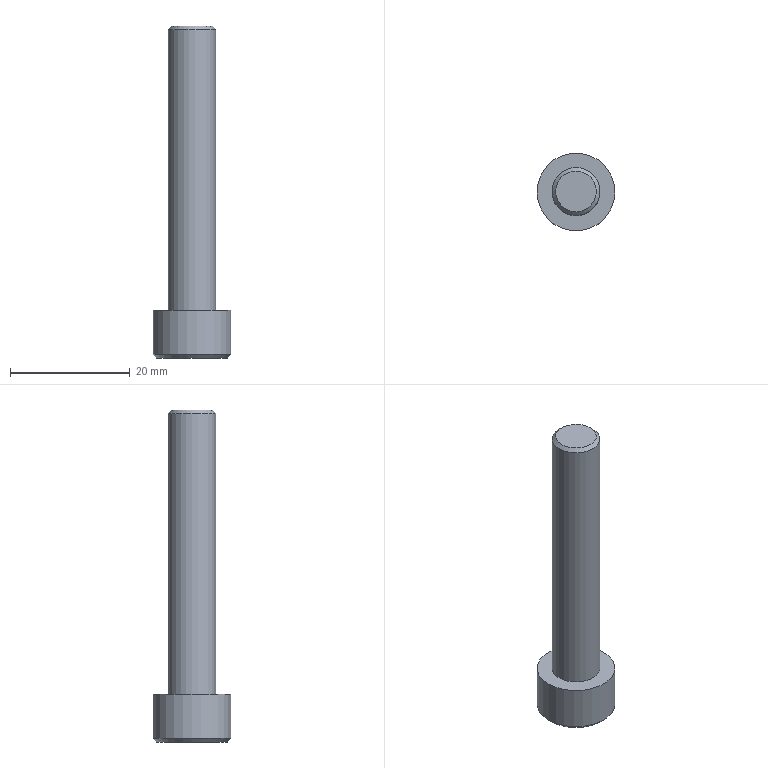Part | NX | features M8.00-55.00 2 | 1 solid | 14 faces | box 13 x 13 x 55.5 mm | volume 3278 mm3 | plane 10 | cylinder 2 | cone 2 | commonest cylinder face diameters 8 x1 13 x1
STEP:
#1=CARTESIAN_POINT('',(19.1,90.,-109.5));
#2=VERTEX_POINT('',#1);
#3=CARTESIAN_POINT('',(25.,90.,-109.5));
#4=DIRECTION('',(0.,0.,-1.));
#5=DIRECTION('',(-1.,0.,0.));
#6=AXIS2_PLACEMENT_3D('',#3,#4,#5);
#7=CIRCLE('',#6,5.9);
#8=EDGE_CURVE('',#2,#2,#7,.T.);
#9=ORIENTED_EDGE('',*,*,#8,.T.);
#10=EDGE_LOOP('',(#9));
#11=FACE_BOUND('',#10,.T.);
#12=CARTESIAN_POINT('',(28.4,91.963,-109.5));
#13=VERTEX_POINT('',#12);
#14=CARTESIAN_POINT('',(28.4,88.037,-109.5));
#15=VERTEX_POINT('',#14);
#16=CARTESIAN_POINT('',(28.4,91.963,-109.5));
#17=DIRECTION('',(0.,-1.,0.));
#18=VECTOR('',#17,1000.);
#19=LINE('',#16,#18);
#20=EDGE_CURVE('',#13,#15,#19,.T.);
#21=ORIENTED_EDGE('',*,*,#20,.F.);
#22=CARTESIAN_POINT('',(25.,93.926,-109.5));
#23=VERTEX_POINT('',#22);
#24=CARTESIAN_POINT('',(25.,93.926,-109.5));
#25=DIRECTION('',(0.866,-0.5,0.));
#26=VECTOR('',#25,1000.);
#27=LINE('',#24,#26);
#28=EDGE_CURVE('',#23,#13,#27,.T.);
#29=ORIENTED_EDGE('',*,*,#28,.F.);
#30=CARTESIAN_POINT('',(21.6,91.963,-109.5));
#31=VERTEX_POINT('',#30);
#32=CARTESIAN_POINT('',(21.6,91.963,-109.5));
#33=DIRECTION('',(0.866,0.5,0.));
#34=VECTOR('',#33,1000.);
#35=LINE('',#32,#34);
#36=EDGE_CURVE('',#31,#23,#35,.T.);
#37=ORIENTED_EDGE('',*,*,#36,.F.);
#38=CARTESIAN_POINT('',(21.6,88.037,-109.5));
#39=VERTEX_POINT('',#38);
#40=CARTESIAN_POINT('',(21.6,88.037,-109.5));
#41=DIRECTION('',(0.,1.,0.));
#42=VECTOR('',#41,1000.);
#43=LINE('',#40,#42);
#44=EDGE_CURVE('',#39,#31,#43,.T.);
#45=ORIENTED_EDGE('',*,*,#44,.F.);
#46=CARTESIAN_POINT('',(25.,86.074,-109.5));
#47=VERTEX_POINT('',#46);
#48=CARTESIAN_POINT('',(25.,86.074,-109.5));
#49=DIRECTION('',(-0.866,0.5,0.));
#50=VECTOR('',#49,1000.);
#51=LINE('',#48,#50);
#52=EDGE_CURVE('',#47,#39,#51,.T.);
#53=ORIENTED_EDGE('',*,*,#52,.F.);
#54=CARTESIAN_POINT('',(28.4,88.037,-109.5));
#55=DIRECTION('',(-0.866,-0.5,0.));
#56=VECTOR('',#55,1000.);
#57=LINE('',#54,#56);
#58=EDGE_CURVE('',#15,#47,#57,.T.);
#59=ORIENTED_EDGE('',*,*,#58,.F.);
#60=EDGE_LOOP('',(#21,#29,#37,#45,#53,#59));
#61=FACE_BOUND('',#60,.T.);
#62=CARTESIAN_POINT('',(25.,90.,-109.5));
#63=DIRECTION('',(0.,0.,-1.));
#64=DIRECTION('',(-1.,0.,0.));
#65=AXIS2_PLACEMENT_3D('',#62,#63,#64);
#66=PLANE('',#65);
#67=ADVANCED_FACE('',(#11,#61),#66,.T.);
#68=CARTESIAN_POINT('',(29.,90.,-101.5));
#69=VERTEX_POINT('',#68);
#70=CARTESIAN_POINT('',(25.,90.,-101.5));
#71=DIRECTION('',(0.,0.,1.));
#72=DIRECTION('',(1.,0.,0.));
#73=AXIS2_PLACEMENT_3D('',#70,#71,#72);
#74=CIRCLE('',#73,4.);
#75=EDGE_CURVE('',#69,#69,#74,.T.);
#76=ORIENTED_EDGE('',*,*,#75,.F.);
#77=EDGE_LOOP('',(#76));
#78=FACE_BOUND('',#77,.T.);
#79=CARTESIAN_POINT('',(31.5,90.,-101.5));
#80=VERTEX_POINT('',#79);
#81=CARTESIAN_POINT('',(25.,90.,-101.5));
#82=DIRECTION('',(0.,0.,-1.));
#83=DIRECTION('',(1.,0.,0.));
#84=AXIS2_PLACEMENT_3D('',#81,#82,#83);
#85=CIRCLE('',#84,6.5);
#86=EDGE_CURVE('',#80,#80,#85,.T.);
#87=ORIENTED_EDGE('',*,*,#86,.F.);
#88=EDGE_LOOP('',(#87));
#89=FACE_BOUND('',#88,.T.);
#90=CARTESIAN_POINT('',(25.,90.,-101.5));
#91=DIRECTION('',(0.,0.,1.));
#92=DIRECTION('',(1.,0.,0.));
#93=AXIS2_PLACEMENT_3D('',#90,#91,#92);
#94=PLANE('',#93);
#95=ADVANCED_FACE('',(#78,#89),#94,.T.);
#96=CARTESIAN_POINT('',(18.5,90.,-108.9));
#97=VERTEX_POINT('',#96);
#98=CARTESIAN_POINT('',(25.,90.,-108.9));
#99=DIRECTION('',(0.,0.,-1.));
#100=DIRECTION('',(-1.,0.,0.));
#101=AXIS2_PLACEMENT_3D('',#98,#99,#100);
#102=CIRCLE('',#101,6.5);
#103=EDGE_CURVE('',#97,#97,#102,.F.);
#104=ORIENTED_EDGE('',*,*,#103,.T.);
#105=EDGE_LOOP('',(#104));
#106=FACE_BOUND('',#105,.T.);
#107=ORIENTED_EDGE('',*,*,#86,.T.);
#108=EDGE_LOOP('',(#107));
#109=FACE_BOUND('',#108,.T.);
#110=CARTESIAN_POINT('',(25.,90.,-101.5));
#111=DIRECTION('',(0.,0.,-1.));
#112=DIRECTION('',(1.,0.,0.));
#113=AXIS2_PLACEMENT_3D('',#110,#111,#112);
#114=CYLINDRICAL_SURFACE('',#113,6.5);
#115=ADVANCED_FACE('',(#106,#109),#114,.T.);
#116=CARTESIAN_POINT('',(28.4,90.,-54.));
#117=VERTEX_POINT('',#116);
#118=CARTESIAN_POINT('',(25.,90.,-54.));
#119=DIRECTION('',(0.,0.,1.));
#120=DIRECTION('',(1.,0.,0.));
#121=AXIS2_PLACEMENT_3D('',#118,#119,#120);
#122=CIRCLE('',#121,3.4);
#123=EDGE_CURVE('',#117,#117,#122,.T.);
#124=ORIENTED_EDGE('',*,*,#123,.T.);
#125=EDGE_LOOP('',(#124));
#126=FACE_BOUND('',#125,.T.);
#127=CARTESIAN_POINT('',(25.,90.,-54.));
#128=DIRECTION('',(0.,0.,1.));
#129=DIRECTION('',(1.,0.,0.));
#130=AXIS2_PLACEMENT_3D('',#127,#128,#129);
#131=PLANE('',#130);
#132=ADVANCED_FACE('',(#126),#131,.T.);
#133=CARTESIAN_POINT('',(29.,90.,-54.6));
#134=VERTEX_POINT('',#133);
#135=CARTESIAN_POINT('',(25.,90.,-54.6));
#136=DIRECTION('',(0.,0.,1.));
#137=DIRECTION('',(1.,0.,0.));
#138=AXIS2_PLACEMENT_3D('',#135,#136,#137);
#139=CIRCLE('',#138,4.);
#140=EDGE_CURVE('',#134,#134,#139,.F.);
#141=ORIENTED_EDGE('',*,*,#140,.T.);
#142=EDGE_LOOP('',(#141));
#143=FACE_BOUND('',#142,.T.);
#144=ORIENTED_EDGE('',*,*,#75,.T.);
#145=EDGE_LOOP('',(#144));
#146=FACE_BOUND('',#145,.T.);
#147=CARTESIAN_POINT('',(25.,90.,-101.5));
#148=DIRECTION('',(0.,0.,1.));
#149=DIRECTION('',(1.,0.,0.));
#150=AXIS2_PLACEMENT_3D('',#147,#148,#149);
#151=CYLINDRICAL_SURFACE('',#150,4.);
#152=ADVANCED_FACE('',(#143,#146),#151,.T.);
#153=ORIENTED_EDGE('',*,*,#58,.T.);
#154=CARTESIAN_POINT('',(25.,86.074,-105.5));
#155=VERTEX_POINT('',#154);
#156=CARTESIAN_POINT('',(25.,86.074,-105.5));
#157=DIRECTION('',(0.,0.,-1.));
#158=VECTOR('',#157,1000.);
#159=LINE('',#156,#158);
#160=EDGE_CURVE('',#47,#155,#159,.F.);
#161=ORIENTED_EDGE('',*,*,#160,.T.);
#162=CARTESIAN_POINT('',(28.4,88.037,-105.5));
#163=VERTEX_POINT('',#162);
#164=CARTESIAN_POINT('',(28.4,88.037,-105.5));
#165=DIRECTION('',(-0.866,-0.5,0.));
#166=VECTOR('',#165,1000.);
#167=LINE('',#164,#166);
#168=EDGE_CURVE('',#155,#163,#167,.F.);
#169=ORIENTED_EDGE('',*,*,#168,.T.);
#170=CARTESIAN_POINT('',(28.4,88.037,-105.5));
#171=DIRECTION('',(0.,0.,-1.));
#172=VECTOR('',#171,1000.);
#173=LINE('',#170,#172);
#174=EDGE_CURVE('',#15,#163,#173,.F.);
#175=ORIENTED_EDGE('',*,*,#174,.F.);
#176=EDGE_LOOP('',(#153,#161,#169,#175));
#177=FACE_BOUND('',#176,.T.);
#178=CARTESIAN_POINT('',(26.7,87.056,-107.5));
#179=DIRECTION('',(0.5,-0.866,0.));
#180=DIRECTION('',(0.866,0.5,0.));
#181=AXIS2_PLACEMENT_3D('',#178,#179,#180);
#182=PLANE('',#181);
#183=ADVANCED_FACE('',(#177),#182,.F.);
#184=ORIENTED_EDGE('',*,*,#20,.T.);
#185=ORIENTED_EDGE('',*,*,#174,.T.);
#186=CARTESIAN_POINT('',(28.4,91.963,-105.5));
#187=VERTEX_POINT('',#186);
#188=CARTESIAN_POINT('',(28.4,91.963,-105.5));
#189=DIRECTION('',(0.,-1.,0.));
#190=VECTOR('',#189,1000.);
#191=LINE('',#188,#190);
#192=EDGE_CURVE('',#163,#187,#191,.F.);
#193=ORIENTED_EDGE('',*,*,#192,.T.);
#194=CARTESIAN_POINT('',(28.4,91.963,-105.5));
#195=DIRECTION('',(0.,0.,-1.));
#196=VECTOR('',#195,1000.);
#197=LINE('',#194,#196);
#198=EDGE_CURVE('',#13,#187,#197,.F.);
#199=ORIENTED_EDGE('',*,*,#198,.F.);
#200=EDGE_LOOP('',(#184,#185,#193,#199));
#201=FACE_BOUND('',#200,.T.);
#202=CARTESIAN_POINT('',(28.4,90.,-107.5));
#203=DIRECTION('',(1.,0.,0.));
#204=DIRECTION('',(0.,0.,-1.));
#205=AXIS2_PLACEMENT_3D('',#202,#203,#204);
#206=PLANE('',#205);
#207=ADVANCED_FACE('',(#201),#206,.F.);
#208=ORIENTED_EDGE('',*,*,#28,.T.);
#209=ORIENTED_EDGE('',*,*,#198,.T.);
#210=CARTESIAN_POINT('',(25.,93.926,-105.5));
#211=VERTEX_POINT('',#210);
#212=CARTESIAN_POINT('',(25.,93.926,-105.5));
#213=DIRECTION('',(0.866,-0.5,0.));
#214=VECTOR('',#213,1000.);
#215=LINE('',#212,#214);
#216=EDGE_CURVE('',#187,#211,#215,.F.);
#217=ORIENTED_EDGE('',*,*,#216,.T.);
#218=CARTESIAN_POINT('',(25.,93.926,-105.5));
#219=DIRECTION('',(0.,0.,-1.));
#220=VECTOR('',#219,1000.);
#221=LINE('',#218,#220);
#222=EDGE_CURVE('',#23,#211,#221,.F.);
#223=ORIENTED_EDGE('',*,*,#222,.F.);
#224=EDGE_LOOP('',(#208,#209,#217,#223));
#225=FACE_BOUND('',#224,.T.);
#226=CARTESIAN_POINT('',(26.7,92.944,-107.5));
#227=DIRECTION('',(0.5,0.866,0.));
#228=DIRECTION('',(-0.866,0.5,0.));
#229=AXIS2_PLACEMENT_3D('',#226,#227,#228);
#230=PLANE('',#229);
#231=ADVANCED_FACE('',(#225),#230,.F.);
#232=ORIENTED_EDGE('',*,*,#36,.T.);
#233=ORIENTED_EDGE('',*,*,#222,.T.);
#234=CARTESIAN_POINT('',(21.6,91.963,-105.5));
#235=VERTEX_POINT('',#234);
#236=CARTESIAN_POINT('',(21.6,91.963,-105.5));
#237=DIRECTION('',(0.866,0.5,0.));
#238=VECTOR('',#237,1000.);
#239=LINE('',#236,#238);
#240=EDGE_CURVE('',#211,#235,#239,.F.);
#241=ORIENTED_EDGE('',*,*,#240,.T.);
#242=CARTESIAN_POINT('',(21.6,91.963,-105.5));
#243=DIRECTION('',(0.,0.,-1.));
#244=VECTOR('',#243,1000.);
#245=LINE('',#242,#244);
#246=EDGE_CURVE('',#31,#235,#245,.F.);
#247=ORIENTED_EDGE('',*,*,#246,.F.);
#248=EDGE_LOOP('',(#232,#233,#241,#247));
#249=FACE_BOUND('',#248,.T.);
#250=CARTESIAN_POINT('',(23.3,92.944,-107.5));
#251=DIRECTION('',(-0.5,0.866,0.));
#252=DIRECTION('',(-0.866,-0.5,0.));
#253=AXIS2_PLACEMENT_3D('',#250,#251,#252);
#254=PLANE('',#253);
#255=ADVANCED_FACE('',(#249),#254,.F.);
#256=ORIENTED_EDGE('',*,*,#44,.T.);
#257=ORIENTED_EDGE('',*,*,#246,.T.);
#258=CARTESIAN_POINT('',(21.6,88.037,-105.5));
#259=VERTEX_POINT('',#258);
#260=CARTESIAN_POINT('',(21.6,88.037,-105.5));
#261=DIRECTION('',(0.,1.,0.));
#262=VECTOR('',#261,1000.);
#263=LINE('',#260,#262);
#264=EDGE_CURVE('',#235,#259,#263,.F.);
#265=ORIENTED_EDGE('',*,*,#264,.T.);
#266=CARTESIAN_POINT('',(21.6,88.037,-105.5));
#267=DIRECTION('',(0.,0.,-1.));
#268=VECTOR('',#267,1000.);
#269=LINE('',#266,#268);
#270=EDGE_CURVE('',#39,#259,#269,.F.);
#271=ORIENTED_EDGE('',*,*,#270,.F.);
#272=EDGE_LOOP('',(#256,#257,#265,#271));
#273=FACE_BOUND('',#272,.T.);
#274=CARTESIAN_POINT('',(21.6,90.,-107.5));
#275=DIRECTION('',(-1.,0.,0.));
#276=DIRECTION('',(0.,0.,1.));
#277=AXIS2_PLACEMENT_3D('',#274,#275,#276);
#278=PLANE('',#277);
#279=ADVANCED_FACE('',(#273),#278,.F.);
#280=ORIENTED_EDGE('',*,*,#52,.T.);
#281=ORIENTED_EDGE('',*,*,#270,.T.);
#282=CARTESIAN_POINT('',(25.,86.074,-105.5));
#283=DIRECTION('',(-0.866,0.5,0.));
#284=VECTOR('',#283,1000.);
#285=LINE('',#282,#284);
#286=EDGE_CURVE('',#259,#155,#285,.F.);
#287=ORIENTED_EDGE('',*,*,#286,.T.);
#288=ORIENTED_EDGE('',*,*,#160,.F.);
#289=EDGE_LOOP('',(#280,#281,#287,#288));
#290=FACE_BOUND('',#289,.T.);
#291=CARTESIAN_POINT('',(23.3,87.056,-107.5));
#292=DIRECTION('',(-0.5,-0.866,0.));
#293=DIRECTION('',(0.866,-0.5,0.));
#294=AXIS2_PLACEMENT_3D('',#291,#292,#293);
#295=PLANE('',#294);
#296=ADVANCED_FACE('',(#290),#295,.F.);
#297=ORIENTED_EDGE('',*,*,#286,.F.);
#298=ORIENTED_EDGE('',*,*,#264,.F.);
#299=ORIENTED_EDGE('',*,*,#240,.F.);
#300=ORIENTED_EDGE('',*,*,#216,.F.);
#301=ORIENTED_EDGE('',*,*,#192,.F.);
#302=ORIENTED_EDGE('',*,*,#168,.F.);
#303=EDGE_LOOP('',(#297,#298,#299,#300,#301,#302));
#304=FACE_BOUND('',#303,.T.);
#305=CARTESIAN_POINT('',(25.,90.,-105.5));
#306=DIRECTION('',(0.,0.,1.));
#307=DIRECTION('',(1.,0.,0.));
#308=AXIS2_PLACEMENT_3D('',#305,#306,#307);
#309=PLANE('',#308);
#310=ADVANCED_FACE('',(#304),#309,.F.);
#311=ORIENTED_EDGE('',*,*,#123,.F.);
#312=EDGE_LOOP('',(#311));
#313=FACE_BOUND('',#312,.T.);
#314=ORIENTED_EDGE('',*,*,#140,.F.);
#315=EDGE_LOOP('',(#314));
#316=FACE_BOUND('',#315,.T.);
#317=CARTESIAN_POINT('',(25.,90.,-54.6));
#318=DIRECTION('',(0.,0.,-1.));
#319=DIRECTION('',(-1.,0.,0.));
#320=AXIS2_PLACEMENT_3D('',#317,#318,#319);
#321=CONICAL_SURFACE('',#320,4.,0.7854);
#322=ADVANCED_FACE('',(#313,#316),#321,.T.);
#323=ORIENTED_EDGE('',*,*,#8,.F.);
#324=EDGE_LOOP('',(#323));
#325=FACE_BOUND('',#324,.T.);
#326=ORIENTED_EDGE('',*,*,#103,.F.);
#327=EDGE_LOOP('',(#326));
#328=FACE_BOUND('',#327,.T.);
#329=CARTESIAN_POINT('',(25.,90.,-108.9));
#330=DIRECTION('',(0.,0.,1.));
#331=DIRECTION('',(1.,0.,0.));
#332=AXIS2_PLACEMENT_3D('',#329,#330,#331);
#333=CONICAL_SURFACE('',#332,6.5,0.7854);
#334=ADVANCED_FACE('',(#325,#328),#333,.T.);
#335=CLOSED_SHELL('',(#67,#95,#115,#132,#152,#183,#207,#231,#255,#279,#296,#310,#322,#334));
#336=MANIFOLD_SOLID_BREP('',#335);
#337=(LENGTH_UNIT()NAMED_UNIT(*)SI_UNIT(.MILLI.,.METRE.));
#338=UNCERTAINTY_MEASURE_WITH_UNIT(LENGTH_MEASURE(0.00001),#337,'','');
#339=(NAMED_UNIT(*)PLANE_ANGLE_UNIT()SI_UNIT($,.RADIAN.));
#340=(NAMED_UNIT(*)SI_UNIT($,.STERADIAN.)SOLID_ANGLE_UNIT());
#341=(GEOMETRIC_REPRESENTATION_CONTEXT(3)GLOBAL_UNCERTAINTY_ASSIGNED_CONTEXT((#338))GLOBAL_UNIT_ASSIGNED_CONTEXT((#337,#339,#340))REPRESENTATION_CONTEXT('',''));
#342=ADVANCED_BREP_SHAPE_REPRESENTATION('',(#336),#341);